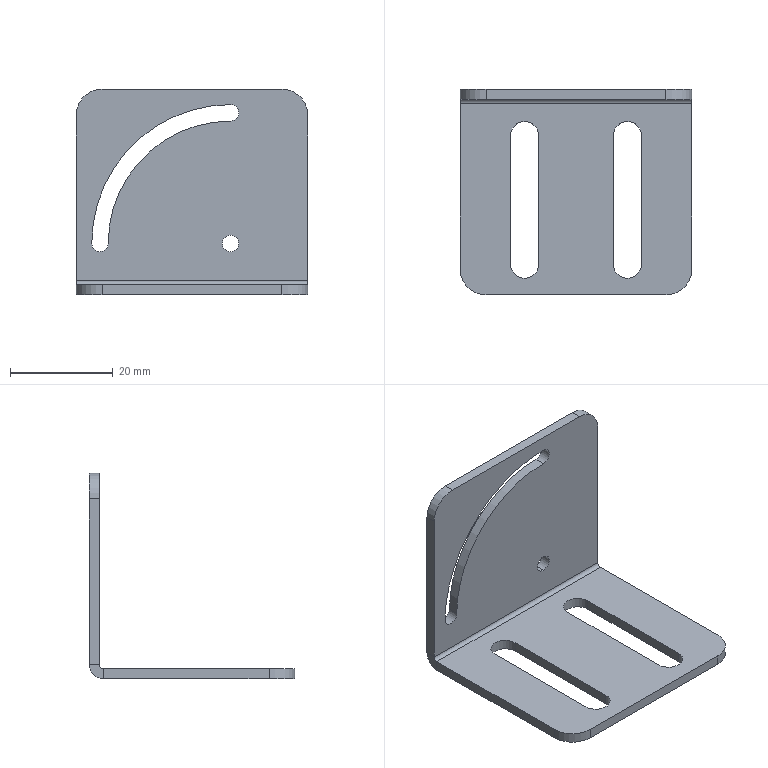Part | SolidWorks | features ICE 2, EdgeFlange 1, Fillet 1, FlatPattern 1, HoleWzd 1, SMBaseFlange 1, SheetMetal 1 | 1 solid | 32 faces | box 45 x 40 x 40 mm | volume 5977 mm3 | cylinder 16 | plane 16 | commonest cylinder face diameters 3.2 x4 5.5 x4 10 x4 1.473 x1 5.473 x1 47.6 x1
STEP:
#1=CARTESIAN_POINT('',(7.5,18.,8.4));
#2=VERTEX_POINT('',#1);
#3=CARTESIAN_POINT('',(7.5,18.,11.6));
#4=VERTEX_POINT('',#3);
#5=CARTESIAN_POINT('',(7.5,18.,10.));
#6=DIRECTION('',(0.,1.,0.));
#7=DIRECTION('',(0.,0.,1.));
#8=AXIS2_PLACEMENT_3D('',#5,#6,#7);
#9=CIRCLE('',#8,1.6);
#10=EDGE_CURVE('',#2,#4,#9,.T.);
#11=ORIENTED_EDGE('',*,*,#10,.F.);
#12=CARTESIAN_POINT('',(7.5,20.,8.4));
#13=VERTEX_POINT('',#12);
#14=CARTESIAN_POINT('',(7.5,20.,8.4));
#15=DIRECTION('',(0.,1.,0.));
#16=VECTOR('',#15,1000.);
#17=LINE('',#14,#16);
#18=EDGE_CURVE('',#2,#13,#17,.T.);
#19=ORIENTED_EDGE('',*,*,#18,.T.);
#20=CARTESIAN_POINT('',(7.5,20.,11.6));
#21=VERTEX_POINT('',#20);
#22=CARTESIAN_POINT('',(7.5,20.,10.));
#23=DIRECTION('',(0.,1.,0.));
#24=DIRECTION('',(0.,0.,1.));
#25=AXIS2_PLACEMENT_3D('',#22,#23,#24);
#26=CIRCLE('',#25,1.6);
#27=EDGE_CURVE('',#13,#21,#26,.T.);
#28=ORIENTED_EDGE('',*,*,#27,.T.);
#29=CARTESIAN_POINT('',(7.5,20.,11.6));
#30=DIRECTION('',(0.,1.,0.));
#31=VECTOR('',#30,1000.);
#32=LINE('',#29,#31);
#33=EDGE_CURVE('',#4,#21,#32,.T.);
#34=ORIENTED_EDGE('',*,*,#33,.F.);
#35=EDGE_LOOP('',(#11,#19,#28,#34));
#36=FACE_OUTER_BOUND('',#35,.T.);
#37=CARTESIAN_POINT('',(7.5,20.,10.));
#38=DIRECTION('',(0.,1.,0.));
#39=DIRECTION('',(0.,0.,1.));
#40=AXIS2_PLACEMENT_3D('',#37,#38,#39);
#41=CYLINDRICAL_SURFACE('',#40,1.6);
#42=ADVANCED_FACE('',(#36),#41,.F.);
#43=CARTESIAN_POINT('',(22.5,-15.,2.));
#44=VERTEX_POINT('',#43);
#45=CARTESIAN_POINT('',(22.5,17.263,2.));
#46=VERTEX_POINT('',#45);
#47=CARTESIAN_POINT('',(22.5,-20.,2.));
#48=DIRECTION('',(0.,1.,0.));
#49=VECTOR('',#48,1000.);
#50=LINE('',#47,#49);
#51=EDGE_CURVE('',#44,#46,#50,.T.);
#52=ORIENTED_EDGE('',*,*,#51,.F.);
#53=CARTESIAN_POINT('',(22.5,-15.,0.));
#54=VERTEX_POINT('',#53);
#55=CARTESIAN_POINT('',(22.5,-15.,2.));
#56=DIRECTION('',(0.,0.,-1.));
#57=VECTOR('',#56,1000.);
#58=LINE('',#55,#57);
#59=EDGE_CURVE('',#44,#54,#58,.T.);
#60=ORIENTED_EDGE('',*,*,#59,.T.);
#61=CARTESIAN_POINT('',(22.5,17.263,0.));
#62=VERTEX_POINT('',#61);
#63=CARTESIAN_POINT('',(22.5,-20.,0.));
#64=DIRECTION('',(0.,1.,0.));
#65=VECTOR('',#64,1000.);
#66=LINE('',#63,#65);
#67=EDGE_CURVE('',#54,#62,#66,.T.);
#68=ORIENTED_EDGE('',*,*,#67,.T.);
#69=CARTESIAN_POINT('',(22.5,17.263,2.));
#70=DIRECTION('',(0.,0.,-1.));
#71=VECTOR('',#70,1000.);
#72=LINE('',#69,#71);
#73=EDGE_CURVE('',#46,#62,#72,.T.);
#74=ORIENTED_EDGE('',*,*,#73,.F.);
#75=EDGE_LOOP('',(#52,#60,#68,#74));
#76=FACE_OUTER_BOUND('',#75,.T.);
#77=CARTESIAN_POINT('',(22.5,-20.,2.));
#78=DIRECTION('',(-1.,0.,0.));
#79=DIRECTION('',(0.,0.,1.));
#80=AXIS2_PLACEMENT_3D('',#77,#78,#79);
#81=PLANE('',#80);
#82=ADVANCED_FACE('',(#76),#81,.F.);
#83=CARTESIAN_POINT('',(-22.5,17.263,0.));
#84=VERTEX_POINT('',#83);
#85=CARTESIAN_POINT('',(-22.5,-15.,0.));
#86=VERTEX_POINT('',#85);
#87=CARTESIAN_POINT('',(-22.5,-20.,0.));
#88=DIRECTION('',(0.,-1.,0.));
#89=VECTOR('',#88,1000.);
#90=LINE('',#87,#89);
#91=EDGE_CURVE('',#84,#86,#90,.T.);
#92=ORIENTED_EDGE('',*,*,#91,.T.);
#93=CARTESIAN_POINT('',(-22.5,-15.,2.));
#94=VERTEX_POINT('',#93);
#95=CARTESIAN_POINT('',(-22.5,-15.,2.));
#96=DIRECTION('',(0.,0.,1.));
#97=VECTOR('',#96,1000.);
#98=LINE('',#95,#97);
#99=EDGE_CURVE('',#86,#94,#98,.T.);
#100=ORIENTED_EDGE('',*,*,#99,.T.);
#101=CARTESIAN_POINT('',(-22.5,17.263,2.));
#102=VERTEX_POINT('',#101);
#103=CARTESIAN_POINT('',(-22.5,-20.,2.));
#104=DIRECTION('',(0.,-1.,0.));
#105=VECTOR('',#104,1000.);
#106=LINE('',#103,#105);
#107=EDGE_CURVE('',#102,#94,#106,.T.);
#108=ORIENTED_EDGE('',*,*,#107,.F.);
#109=CARTESIAN_POINT('',(-22.5,17.263,2.));
#110=DIRECTION('',(0.,0.,-1.));
#111=VECTOR('',#110,1000.);
#112=LINE('',#109,#111);
#113=EDGE_CURVE('',#102,#84,#112,.T.);
#114=ORIENTED_EDGE('',*,*,#113,.T.);
#115=EDGE_LOOP('',(#92,#100,#108,#114));
#116=FACE_OUTER_BOUND('',#115,.T.);
#117=CARTESIAN_POINT('',(-22.5,-20.,2.));
#118=DIRECTION('',(1.,0.,0.));
#119=DIRECTION('',(0.,0.,-1.));
#120=AXIS2_PLACEMENT_3D('',#117,#118,#119);
#121=PLANE('',#120);
#122=ADVANCED_FACE('',(#116),#121,.F.);
#123=CARTESIAN_POINT('',(-12.75,11.,2.));
#124=VERTEX_POINT('',#123);
#125=CARTESIAN_POINT('',(-12.75,-14.,2.));
#126=VERTEX_POINT('',#125);
#127=CARTESIAN_POINT('',(-12.75,11.,2.));
#128=DIRECTION('',(0.,-1.,0.));
#129=VECTOR('',#128,1000.);
#130=LINE('',#127,#129);
#131=EDGE_CURVE('',#124,#126,#130,.T.);
#132=ORIENTED_EDGE('',*,*,#131,.F.);
#133=CARTESIAN_POINT('',(-7.25,11.,2.));
#134=VERTEX_POINT('',#133);
#135=CARTESIAN_POINT('',(-10.,11.,2.));
#136=DIRECTION('',(0.,0.,1.));
#137=DIRECTION('',(1.,0.,0.));
#138=AXIS2_PLACEMENT_3D('',#135,#136,#137);
#139=CIRCLE('',#138,2.75);
#140=EDGE_CURVE('',#134,#124,#139,.T.);
#141=ORIENTED_EDGE('',*,*,#140,.F.);
#142=CARTESIAN_POINT('',(-7.25,-14.,2.));
#143=VERTEX_POINT('',#142);
#144=CARTESIAN_POINT('',(-7.25,11.,2.));
#145=DIRECTION('',(0.,1.,0.));
#146=VECTOR('',#145,1000.);
#147=LINE('',#144,#146);
#148=EDGE_CURVE('',#143,#134,#147,.T.);
#149=ORIENTED_EDGE('',*,*,#148,.F.);
#150=CARTESIAN_POINT('',(-10.,-14.,2.));
#151=DIRECTION('',(0.,0.,1.));
#152=DIRECTION('',(1.,0.,0.));
#153=AXIS2_PLACEMENT_3D('',#150,#151,#152);
#154=CIRCLE('',#153,2.75);
#155=EDGE_CURVE('',#126,#143,#154,.T.);
#156=ORIENTED_EDGE('',*,*,#155,.F.);
#157=EDGE_LOOP('',(#132,#141,#149,#156));
#158=FACE_BOUND('',#157,.T.);
#159=CARTESIAN_POINT('',(7.25,11.,2.));
#160=VERTEX_POINT('',#159);
#161=CARTESIAN_POINT('',(7.25,-14.,2.));
#162=VERTEX_POINT('',#161);
#163=CARTESIAN_POINT('',(7.25,11.,2.));
#164=DIRECTION('',(0.,-1.,0.));
#165=VECTOR('',#164,1000.);
#166=LINE('',#163,#165);
#167=EDGE_CURVE('',#160,#162,#166,.T.);
#168=ORIENTED_EDGE('',*,*,#167,.F.);
#169=CARTESIAN_POINT('',(12.75,11.,2.));
#170=VERTEX_POINT('',#169);
#171=CARTESIAN_POINT('',(10.,11.,2.));
#172=DIRECTION('',(0.,0.,1.));
#173=DIRECTION('',(1.,0.,0.));
#174=AXIS2_PLACEMENT_3D('',#171,#172,#173);
#175=CIRCLE('',#174,2.75);
#176=EDGE_CURVE('',#170,#160,#175,.T.);
#177=ORIENTED_EDGE('',*,*,#176,.F.);
#178=CARTESIAN_POINT('',(12.75,-14.,2.));
#179=VERTEX_POINT('',#178);
#180=CARTESIAN_POINT('',(12.75,11.,2.));
#181=DIRECTION('',(0.,1.,0.));
#182=VECTOR('',#181,1000.);
#183=LINE('',#180,#182);
#184=EDGE_CURVE('',#179,#170,#183,.T.);
#185=ORIENTED_EDGE('',*,*,#184,.F.);
#186=CARTESIAN_POINT('',(10.,-14.,2.));
#187=DIRECTION('',(0.,0.,1.));
#188=DIRECTION('',(1.,0.,0.));
#189=AXIS2_PLACEMENT_3D('',#186,#187,#188);
#190=CIRCLE('',#189,2.75);
#191=EDGE_CURVE('',#162,#179,#190,.T.);
#192=ORIENTED_EDGE('',*,*,#191,.F.);
#193=EDGE_LOOP('',(#168,#177,#185,#192));
#194=FACE_BOUND('',#193,.T.);
#195=ORIENTED_EDGE('',*,*,#107,.T.);
#196=CARTESIAN_POINT('',(-17.5,-20.,2.));
#197=VERTEX_POINT('',#196);
#198=CARTESIAN_POINT('',(-17.5,-15.,2.));
#199=DIRECTION('',(0.,0.,1.));
#200=DIRECTION('',(-1.,0.,0.));
#201=AXIS2_PLACEMENT_3D('',#198,#199,#200);
#202=CIRCLE('',#201,5.);
#203=EDGE_CURVE('',#94,#197,#202,.T.);
#204=ORIENTED_EDGE('',*,*,#203,.T.);
#205=CARTESIAN_POINT('',(17.5,-20.,2.));
#206=VERTEX_POINT('',#205);
#207=CARTESIAN_POINT('',(-22.5,-20.,2.));
#208=DIRECTION('',(1.,0.,0.));
#209=VECTOR('',#208,1000.);
#210=LINE('',#207,#209);
#211=EDGE_CURVE('',#197,#206,#210,.T.);
#212=ORIENTED_EDGE('',*,*,#211,.T.);
#213=CARTESIAN_POINT('',(17.5,-15.,2.));
#214=DIRECTION('',(0.,0.,1.));
#215=DIRECTION('',(-1.,0.,0.));
#216=AXIS2_PLACEMENT_3D('',#213,#214,#215);
#217=CIRCLE('',#216,5.);
#218=EDGE_CURVE('',#206,#44,#217,.T.);
#219=ORIENTED_EDGE('',*,*,#218,.T.);
#220=ORIENTED_EDGE('',*,*,#51,.T.);
#221=CARTESIAN_POINT('',(-22.5,17.263,2.));
#222=DIRECTION('',(1.,0.,0.));
#223=VECTOR('',#222,1000.);
#224=LINE('',#221,#223);
#225=EDGE_CURVE('',#102,#46,#224,.T.);
#226=ORIENTED_EDGE('',*,*,#225,.F.);
#227=EDGE_LOOP('',(#195,#204,#212,#219,#220,#226));
#228=FACE_OUTER_BOUND('',#227,.T.);
#229=CARTESIAN_POINT('',(0.,0.,2.));
#230=DIRECTION('',(0.,0.,-1.));
#231=DIRECTION('',(-1.,0.,0.));
#232=AXIS2_PLACEMENT_3D('',#229,#230,#231);
#233=PLANE('',#232);
#234=ADVANCED_FACE('',(#158,#194,#228),#233,.F.);
#235=CARTESIAN_POINT('',(-7.25,11.,0.));
#236=VERTEX_POINT('',#235);
#237=CARTESIAN_POINT('',(-12.75,11.,0.));
#238=VERTEX_POINT('',#237);
#239=CARTESIAN_POINT('',(-10.,11.,0.));
#240=DIRECTION('',(0.,0.,1.));
#241=DIRECTION('',(1.,0.,0.));
#242=AXIS2_PLACEMENT_3D('',#239,#240,#241);
#243=CIRCLE('',#242,2.75);
#244=EDGE_CURVE('',#236,#238,#243,.T.);
#245=ORIENTED_EDGE('',*,*,#244,.T.);
#246=CARTESIAN_POINT('',(-12.75,-14.,0.));
#247=VERTEX_POINT('',#246);
#248=CARTESIAN_POINT('',(-12.75,11.,0.));
#249=DIRECTION('',(0.,-1.,0.));
#250=VECTOR('',#249,1000.);
#251=LINE('',#248,#250);
#252=EDGE_CURVE('',#238,#247,#251,.T.);
#253=ORIENTED_EDGE('',*,*,#252,.T.);
#254=CARTESIAN_POINT('',(-7.25,-14.,0.));
#255=VERTEX_POINT('',#254);
#256=CARTESIAN_POINT('',(-10.,-14.,0.));
#257=DIRECTION('',(0.,0.,1.));
#258=DIRECTION('',(1.,0.,0.));
#259=AXIS2_PLACEMENT_3D('',#256,#257,#258);
#260=CIRCLE('',#259,2.75);
#261=EDGE_CURVE('',#247,#255,#260,.T.);
#262=ORIENTED_EDGE('',*,*,#261,.T.);
#263=CARTESIAN_POINT('',(-7.25,11.,0.));
#264=DIRECTION('',(0.,1.,0.));
#265=VECTOR('',#264,1000.);
#266=LINE('',#263,#265);
#267=EDGE_CURVE('',#255,#236,#266,.T.);
#268=ORIENTED_EDGE('',*,*,#267,.T.);
#269=EDGE_LOOP('',(#245,#253,#262,#268));
#270=FACE_BOUND('',#269,.T.);
#271=CARTESIAN_POINT('',(12.75,11.,0.));
#272=VERTEX_POINT('',#271);
#273=CARTESIAN_POINT('',(7.25,11.,0.));
#274=VERTEX_POINT('',#273);
#275=CARTESIAN_POINT('',(10.,11.,0.));
#276=DIRECTION('',(0.,0.,1.));
#277=DIRECTION('',(1.,0.,0.));
#278=AXIS2_PLACEMENT_3D('',#275,#276,#277);
#279=CIRCLE('',#278,2.75);
#280=EDGE_CURVE('',#272,#274,#279,.T.);
#281=ORIENTED_EDGE('',*,*,#280,.T.);
#282=CARTESIAN_POINT('',(7.25,-14.,0.));
#283=VERTEX_POINT('',#282);
#284=CARTESIAN_POINT('',(7.25,11.,0.));
#285=DIRECTION('',(0.,-1.,0.));
#286=VECTOR('',#285,1000.);
#287=LINE('',#284,#286);
#288=EDGE_CURVE('',#274,#283,#287,.T.);
#289=ORIENTED_EDGE('',*,*,#288,.T.);
#290=CARTESIAN_POINT('',(12.75,-14.,0.));
#291=VERTEX_POINT('',#290);
#292=CARTESIAN_POINT('',(10.,-14.,0.));
#293=DIRECTION('',(0.,0.,1.));
#294=DIRECTION('',(1.,0.,0.));
#295=AXIS2_PLACEMENT_3D('',#292,#293,#294);
#296=CIRCLE('',#295,2.75);
#297=EDGE_CURVE('',#283,#291,#296,.T.);
#298=ORIENTED_EDGE('',*,*,#297,.T.);
#299=CARTESIAN_POINT('',(12.75,11.,0.));
#300=DIRECTION('',(0.,1.,0.));
#301=VECTOR('',#300,1000.);
#302=LINE('',#299,#301);
#303=EDGE_CURVE('',#291,#272,#302,.T.);
#304=ORIENTED_EDGE('',*,*,#303,.T.);
#305=EDGE_LOOP('',(#281,#289,#298,#304));
#306=FACE_BOUND('',#305,.T.);
#307=CARTESIAN_POINT('',(-17.5,-20.,0.));
#308=VERTEX_POINT('',#307);
#309=CARTESIAN_POINT('',(17.5,-20.,0.));
#310=VERTEX_POINT('',#309);
#311=CARTESIAN_POINT('',(-22.5,-20.,0.));
#312=DIRECTION('',(1.,0.,0.));
#313=VECTOR('',#312,1000.);
#314=LINE('',#311,#313);
#315=EDGE_CURVE('',#308,#310,#314,.T.);
#316=ORIENTED_EDGE('',*,*,#315,.F.);
#317=CARTESIAN_POINT('',(-17.5,-15.,0.));
#318=DIRECTION('',(0.,0.,-1.));
#319=DIRECTION('',(-1.,0.,0.));
#320=AXIS2_PLACEMENT_3D('',#317,#318,#319);
#321=CIRCLE('',#320,5.);
#322=EDGE_CURVE('',#308,#86,#321,.T.);
#323=ORIENTED_EDGE('',*,*,#322,.T.);
#324=ORIENTED_EDGE('',*,*,#91,.F.);
#325=CARTESIAN_POINT('',(-22.5,17.263,0.));
#326=DIRECTION('',(1.,0.,0.));
#327=VECTOR('',#326,1000.);
#328=LINE('',#325,#327);
#329=EDGE_CURVE('',#84,#62,#328,.T.);
#330=ORIENTED_EDGE('',*,*,#329,.T.);
#331=ORIENTED_EDGE('',*,*,#67,.F.);
#332=CARTESIAN_POINT('',(17.5,-15.,0.));
#333=DIRECTION('',(0.,0.,-1.));
#334=DIRECTION('',(-1.,0.,0.));
#335=AXIS2_PLACEMENT_3D('',#332,#333,#334);
#336=CIRCLE('',#335,5.);
#337=EDGE_CURVE('',#54,#310,#336,.T.);
#338=ORIENTED_EDGE('',*,*,#337,.T.);
#339=EDGE_LOOP('',(#316,#323,#324,#330,#331,#338));
#340=FACE_OUTER_BOUND('',#339,.T.);
#341=CARTESIAN_POINT('',(0.,0.,0.));
#342=DIRECTION('',(0.,0.,-1.));
#343=DIRECTION('',(-1.,0.,0.));
#344=AXIS2_PLACEMENT_3D('',#341,#342,#343);
#345=PLANE('',#344);
#346=ADVANCED_FACE('',(#270,#306,#340),#345,.T.);
#347=ORIENTED_EDGE('',*,*,#211,.F.);
#348=CARTESIAN_POINT('',(-17.5,-20.,2.));
#349=DIRECTION('',(0.,0.,-1.));
#350=VECTOR('',#349,1000.);
#351=LINE('',#348,#350);
#352=EDGE_CURVE('',#197,#308,#351,.T.);
#353=ORIENTED_EDGE('',*,*,#352,.T.);
#354=ORIENTED_EDGE('',*,*,#315,.T.);
#355=CARTESIAN_POINT('',(17.5,-20.,2.));
#356=DIRECTION('',(0.,0.,1.));
#357=VECTOR('',#356,1000.);
#358=LINE('',#355,#357);
#359=EDGE_CURVE('',#310,#206,#358,.T.);
#360=ORIENTED_EDGE('',*,*,#359,.T.);
#361=EDGE_LOOP('',(#347,#353,#354,#360));
#362=FACE_OUTER_BOUND('',#361,.T.);
#363=CARTESIAN_POINT('',(-22.5,-20.,2.));
#364=DIRECTION('',(0.,1.,0.));
#365=DIRECTION('',(0.,0.,1.));
#366=AXIS2_PLACEMENT_3D('',#363,#364,#365);
#367=PLANE('',#366);
#368=ADVANCED_FACE('',(#362),#367,.F.);
#369=CARTESIAN_POINT('',(22.5,18.,2.737));
#370=VERTEX_POINT('',#369);
#371=CARTESIAN_POINT('',(22.5,20.,2.737));
#372=VERTEX_POINT('',#371);
#373=CARTESIAN_POINT('',(22.5,20.,2.737));
#374=DIRECTION('',(0.,1.,0.));
#375=VECTOR('',#374,1000.);
#376=LINE('',#373,#375);
#377=EDGE_CURVE('',#370,#372,#376,.T.);
#378=ORIENTED_EDGE('',*,*,#377,.F.);
#379=CARTESIAN_POINT('',(22.5,17.263,2.737));
#380=DIRECTION('',(1.,0.,0.));
#381=DIRECTION('',(0.,0.,1.));
#382=AXIS2_PLACEMENT_3D('',#379,#380,#381);
#383=CIRCLE('',#382,0.7366);
#384=EDGE_CURVE('',#46,#370,#383,.T.);
#385=ORIENTED_EDGE('',*,*,#384,.F.);
#386=ORIENTED_EDGE('',*,*,#73,.T.);
#387=CARTESIAN_POINT('',(22.5,17.263,2.737));
#388=DIRECTION('',(1.,0.,0.));
#389=DIRECTION('',(0.,0.,1.));
#390=AXIS2_PLACEMENT_3D('',#387,#388,#389);
#391=CIRCLE('',#390,2.737);
#392=EDGE_CURVE('',#62,#372,#391,.T.);
#393=ORIENTED_EDGE('',*,*,#392,.T.);
#394=EDGE_LOOP('',(#378,#385,#386,#393));
#395=FACE_OUTER_BOUND('',#394,.T.);
#396=CARTESIAN_POINT('',(22.5,17.263,2.737));
#397=DIRECTION('',(1.,0.,0.));
#398=DIRECTION('',(0.,0.,-1.));
#399=AXIS2_PLACEMENT_3D('',#396,#397,#398);
#400=PLANE('',#399);
#401=ADVANCED_FACE('',(#395),#400,.T.);
#402=CARTESIAN_POINT('',(-22.5,18.,2.737));
#403=VERTEX_POINT('',#402);
#404=CARTESIAN_POINT('',(-22.5,17.263,2.737));
#405=DIRECTION('',(-1.,0.,0.));
#406=DIRECTION('',(0.,0.,1.));
#407=AXIS2_PLACEMENT_3D('',#404,#405,#406);
#408=CIRCLE('',#407,0.7366);
#409=EDGE_CURVE('',#403,#102,#408,.T.);
#410=ORIENTED_EDGE('',*,*,#409,.F.);
#411=CARTESIAN_POINT('',(-22.5,20.,2.737));
#412=VERTEX_POINT('',#411);
#413=CARTESIAN_POINT('',(-22.5,18.,2.737));
#414=DIRECTION('',(0.,1.,0.));
#415=VECTOR('',#414,1000.);
#416=LINE('',#413,#415);
#417=EDGE_CURVE('',#403,#412,#416,.T.);
#418=ORIENTED_EDGE('',*,*,#417,.T.);
#419=CARTESIAN_POINT('',(-22.5,17.263,2.737));
#420=DIRECTION('',(-1.,0.,0.));
#421=DIRECTION('',(0.,0.,1.));
#422=AXIS2_PLACEMENT_3D('',#419,#420,#421);
#423=CIRCLE('',#422,2.737);
#424=EDGE_CURVE('',#412,#84,#423,.T.);
#425=ORIENTED_EDGE('',*,*,#424,.T.);
#426=ORIENTED_EDGE('',*,*,#113,.F.);
#427=EDGE_LOOP('',(#410,#418,#425,#426));
#428=FACE_OUTER_BOUND('',#427,.T.);
#429=CARTESIAN_POINT('',(-22.5,17.263,2.737));
#430=DIRECTION('',(1.,0.,0.));
#431=DIRECTION('',(0.,0.,-1.));
#432=AXIS2_PLACEMENT_3D('',#429,#430,#431);
#433=PLANE('',#432);
#434=ADVANCED_FACE('',(#428),#433,.F.);
#435=ORIENTED_EDGE('',*,*,#329,.F.);
#436=ORIENTED_EDGE('',*,*,#424,.F.);
#437=CARTESIAN_POINT('',(0.,20.,2.737));
#438=DIRECTION('',(-1.,0.,0.));
#439=VECTOR('',#438,1000.);
#440=LINE('',#437,#439);
#441=EDGE_CURVE('',#372,#412,#440,.T.);
#442=ORIENTED_EDGE('',*,*,#441,.F.);
#443=ORIENTED_EDGE('',*,*,#392,.F.);
#444=EDGE_LOOP('',(#435,#436,#442,#443));
#445=FACE_OUTER_BOUND('',#444,.T.);
#446=CARTESIAN_POINT('',(-22.5,17.263,2.737));
#447=DIRECTION('',(-1.,0.,0.));
#448=DIRECTION('',(0.,1.,0.));
#449=AXIS2_PLACEMENT_3D('',#446,#447,#448);
#450=CYLINDRICAL_SURFACE('',#449,2.737);
#451=ADVANCED_FACE('',(#445),#450,.T.);
#452=ORIENTED_EDGE('',*,*,#225,.T.);
#453=ORIENTED_EDGE('',*,*,#384,.T.);
#454=CARTESIAN_POINT('',(22.5,18.,2.737));
#455=DIRECTION('',(-1.,0.,0.));
#456=VECTOR('',#455,1000.);
#457=LINE('',#454,#456);
#458=EDGE_CURVE('',#370,#403,#457,.T.);
#459=ORIENTED_EDGE('',*,*,#458,.T.);
#460=ORIENTED_EDGE('',*,*,#409,.T.);
#461=EDGE_LOOP('',(#452,#453,#459,#460));
#462=FACE_OUTER_BOUND('',#461,.T.);
#463=CARTESIAN_POINT('',(-22.5,17.263,2.737));
#464=DIRECTION('',(-1.,0.,0.));
#465=DIRECTION('',(0.,1.,0.));
#466=AXIS2_PLACEMENT_3D('',#463,#464,#465);
#467=CYLINDRICAL_SURFACE('',#466,0.7366);
#468=ADVANCED_FACE('',(#462),#467,.F.);
#469=CARTESIAN_POINT('',(-22.5,18.,35.));
#470=VERTEX_POINT('',#469);
#471=CARTESIAN_POINT('',(-22.5,18.,0.));
#472=DIRECTION('',(0.,0.,-1.));
#473=VECTOR('',#472,1000.);
#474=LINE('',#471,#473);
#475=EDGE_CURVE('',#470,#403,#474,.T.);
#476=ORIENTED_EDGE('',*,*,#475,.F.);
#477=CARTESIAN_POINT('',(-22.5,20.,35.));
#478=VERTEX_POINT('',#477);
#479=CARTESIAN_POINT('',(-22.5,20.,35.));
#480=DIRECTION('',(0.,1.,0.));
#481=VECTOR('',#480,1000.);
#482=LINE('',#479,#481);
#483=EDGE_CURVE('',#470,#478,#482,.T.);
#484=ORIENTED_EDGE('',*,*,#483,.T.);
#485=CARTESIAN_POINT('',(-22.5,20.,2.));
#486=DIRECTION('',(0.,0.,-1.));
#487=VECTOR('',#486,1000.);
#488=LINE('',#485,#487);
#489=EDGE_CURVE('',#478,#412,#488,.T.);
#490=ORIENTED_EDGE('',*,*,#489,.T.);
#491=ORIENTED_EDGE('',*,*,#417,.F.);
#492=EDGE_LOOP('',(#476,#484,#490,#491));
#493=FACE_OUTER_BOUND('',#492,.T.);
#494=CARTESIAN_POINT('',(-22.5,20.,2.));
#495=DIRECTION('',(-1.,0.,0.));
#496=DIRECTION('',(0.,0.,1.));
#497=AXIS2_PLACEMENT_3D('',#494,#495,#496);
#498=PLANE('',#497);
#499=ADVANCED_FACE('',(#493),#498,.T.);
#500=CARTESIAN_POINT('',(22.5,20.,35.));
#501=VERTEX_POINT('',#500);
#502=CARTESIAN_POINT('',(22.5,20.,40.));
#503=DIRECTION('',(0.,0.,1.));
#504=VECTOR('',#503,1000.);
#505=LINE('',#502,#504);
#506=EDGE_CURVE('',#372,#501,#505,.T.);
#507=ORIENTED_EDGE('',*,*,#506,.T.);
#508=CARTESIAN_POINT('',(22.5,18.,35.));
#509=VERTEX_POINT('',#508);
#510=CARTESIAN_POINT('',(22.5,20.,35.));
#511=DIRECTION('',(0.,-1.,0.));
#512=VECTOR('',#511,1000.);
#513=LINE('',#510,#512);
#514=EDGE_CURVE('',#501,#509,#513,.T.);
#515=ORIENTED_EDGE('',*,*,#514,.T.);
#516=CARTESIAN_POINT('',(22.5,18.,0.));
#517=DIRECTION('',(0.,0.,1.));
#518=VECTOR('',#517,1000.);
#519=LINE('',#516,#518);
#520=EDGE_CURVE('',#370,#509,#519,.T.);
#521=ORIENTED_EDGE('',*,*,#520,.F.);
#522=ORIENTED_EDGE('',*,*,#377,.T.);
#523=EDGE_LOOP('',(#507,#515,#521,#522));
#524=FACE_OUTER_BOUND('',#523,.T.);
#525=CARTESIAN_POINT('',(22.5,20.,40.));
#526=DIRECTION('',(1.,0.,0.));
#527=DIRECTION('',(0.,0.,-1.));
#528=AXIS2_PLACEMENT_3D('',#525,#526,#527);
#529=PLANE('',#528);
#530=ADVANCED_FACE('',(#524),#529,.T.);
#531=CARTESIAN_POINT('',(-16.3,20.,10.));
#532=VERTEX_POINT('',#531);
#533=CARTESIAN_POINT('',(-19.5,20.,10.));
#534=VERTEX_POINT('',#533);
#535=CARTESIAN_POINT('',(-17.9,20.,10.));
#536=DIRECTION('',(0.,1.,0.));
#537=DIRECTION('',(0.,0.,1.));
#538=AXIS2_PLACEMENT_3D('',#535,#536,#537);
#539=CIRCLE('',#538,1.6);
#540=EDGE_CURVE('',#532,#534,#539,.T.);
#541=ORIENTED_EDGE('',*,*,#540,.F.);
#542=CARTESIAN_POINT('',(7.5,20.,33.8));
#543=VERTEX_POINT('',#542);
#544=CARTESIAN_POINT('',(7.5,20.,10.));
#545=DIRECTION('',(0.,-1.,0.));
#546=DIRECTION('',(0.,0.,1.));
#547=AXIS2_PLACEMENT_3D('',#544,#545,#546);
#548=CIRCLE('',#547,23.8);
#549=EDGE_CURVE('',#543,#532,#548,.T.);
#550=ORIENTED_EDGE('',*,*,#549,.F.);
#551=CARTESIAN_POINT('',(7.5,20.,37.));
#552=VERTEX_POINT('',#551);
#553=CARTESIAN_POINT('',(7.5,20.,35.4));
#554=DIRECTION('',(0.,1.,0.));
#555=DIRECTION('',(0.,0.,1.));
#556=AXIS2_PLACEMENT_3D('',#553,#554,#555);
#557=CIRCLE('',#556,1.6);
#558=EDGE_CURVE('',#552,#543,#557,.T.);
#559=ORIENTED_EDGE('',*,*,#558,.F.);
#560=CARTESIAN_POINT('',(7.5,20.,10.));
#561=DIRECTION('',(0.,1.,0.));
#562=DIRECTION('',(0.,0.,1.));
#563=AXIS2_PLACEMENT_3D('',#560,#561,#562);
#564=CIRCLE('',#563,27.);
#565=EDGE_CURVE('',#534,#552,#564,.T.);
#566=ORIENTED_EDGE('',*,*,#565,.F.);
#567=EDGE_LOOP('',(#541,#550,#559,#566));
#568=FACE_BOUND('',#567,.T.);
#569=CARTESIAN_POINT('',(7.5,20.,10.));
#570=DIRECTION('',(0.,1.,0.));
#571=DIRECTION('',(0.,0.,1.));
#572=AXIS2_PLACEMENT_3D('',#569,#570,#571);
#573=CIRCLE('',#572,1.6);
#574=EDGE_CURVE('',#21,#13,#573,.T.);
#575=ORIENTED_EDGE('',*,*,#574,.F.);
#576=ORIENTED_EDGE('',*,*,#27,.F.);
#577=EDGE_LOOP('',(#575,#576));
#578=FACE_BOUND('',#577,.T.);
#579=CARTESIAN_POINT('',(17.5,20.,40.));
#580=VERTEX_POINT('',#579);
#581=CARTESIAN_POINT('',(-17.5,20.,40.));
#582=VERTEX_POINT('',#581);
#583=CARTESIAN_POINT('',(-22.5,20.,40.));
#584=DIRECTION('',(-1.,0.,0.));
#585=VECTOR('',#584,1000.);
#586=LINE('',#583,#585);
#587=EDGE_CURVE('',#580,#582,#586,.T.);
#588=ORIENTED_EDGE('',*,*,#587,.F.);
#589=CARTESIAN_POINT('',(17.5,20.,35.));
#590=DIRECTION('',(0.,1.,0.));
#591=DIRECTION('',(0.,0.,1.));
#592=AXIS2_PLACEMENT_3D('',#589,#590,#591);
#593=CIRCLE('',#592,5.);
#594=EDGE_CURVE('',#580,#501,#593,.T.);
#595=ORIENTED_EDGE('',*,*,#594,.T.);
#596=ORIENTED_EDGE('',*,*,#506,.F.);
#597=ORIENTED_EDGE('',*,*,#441,.T.);
#598=ORIENTED_EDGE('',*,*,#489,.F.);
#599=CARTESIAN_POINT('',(-17.5,20.,35.));
#600=DIRECTION('',(0.,1.,0.));
#601=DIRECTION('',(0.,0.,1.));
#602=AXIS2_PLACEMENT_3D('',#599,#600,#601);
#603=CIRCLE('',#602,5.);
#604=EDGE_CURVE('',#478,#582,#603,.T.);
#605=ORIENTED_EDGE('',*,*,#604,.T.);
#606=EDGE_LOOP('',(#588,#595,#596,#597,#598,#605));
#607=FACE_OUTER_BOUND('',#606,.T.);
#608=CARTESIAN_POINT('',(0.,20.,0.));
#609=DIRECTION('',(0.,1.,0.));
#610=DIRECTION('',(0.,0.,1.));
#611=AXIS2_PLACEMENT_3D('',#608,#609,#610);
#612=PLANE('',#611);
#613=ADVANCED_FACE('',(#568,#578,#607),#612,.T.);
#614=CARTESIAN_POINT('',(-16.3,18.,10.));
#615=VERTEX_POINT('',#614);
#616=CARTESIAN_POINT('',(7.5,18.,33.8));
#617=VERTEX_POINT('',#616);
#618=CARTESIAN_POINT('',(7.5,18.,10.));
#619=DIRECTION('',(0.,1.,0.));
#620=DIRECTION('',(0.,0.,1.));
#621=AXIS2_PLACEMENT_3D('',#618,#619,#620);
#622=CIRCLE('',#621,23.8);
#623=EDGE_CURVE('',#615,#617,#622,.T.);
#624=ORIENTED_EDGE('',*,*,#623,.F.);
#625=CARTESIAN_POINT('',(-19.5,18.,10.));
#626=VERTEX_POINT('',#625);
#627=CARTESIAN_POINT('',(-17.9,18.,10.));
#628=DIRECTION('',(0.,-1.,0.));
#629=DIRECTION('',(0.,0.,1.));
#630=AXIS2_PLACEMENT_3D('',#627,#628,#629);
#631=CIRCLE('',#630,1.6);
#632=EDGE_CURVE('',#626,#615,#631,.T.);
#633=ORIENTED_EDGE('',*,*,#632,.F.);
#634=CARTESIAN_POINT('',(7.5,18.,37.));
#635=VERTEX_POINT('',#634);
#636=CARTESIAN_POINT('',(7.5,18.,10.));
#637=DIRECTION('',(0.,-1.,0.));
#638=DIRECTION('',(0.,0.,1.));
#639=AXIS2_PLACEMENT_3D('',#636,#637,#638);
#640=CIRCLE('',#639,27.);
#641=EDGE_CURVE('',#635,#626,#640,.T.);
#642=ORIENTED_EDGE('',*,*,#641,.F.);
#643=CARTESIAN_POINT('',(7.5,18.,35.4));
#644=DIRECTION('',(0.,-1.,0.));
#645=DIRECTION('',(0.,0.,1.));
#646=AXIS2_PLACEMENT_3D('',#643,#644,#645);
#647=CIRCLE('',#646,1.6);
#648=EDGE_CURVE('',#617,#635,#647,.T.);
#649=ORIENTED_EDGE('',*,*,#648,.F.);
#650=EDGE_LOOP('',(#624,#633,#642,#649));
#651=FACE_BOUND('',#650,.T.);
#652=CARTESIAN_POINT('',(7.5,18.,10.));
#653=DIRECTION('',(0.,1.,0.));
#654=DIRECTION('',(0.,0.,1.));
#655=AXIS2_PLACEMENT_3D('',#652,#653,#654);
#656=CIRCLE('',#655,1.6);
#657=EDGE_CURVE('',#4,#2,#656,.T.);
#658=ORIENTED_EDGE('',*,*,#657,.T.);
#659=ORIENTED_EDGE('',*,*,#10,.T.);
#660=EDGE_LOOP('',(#658,#659));
#661=FACE_BOUND('',#660,.T.);
#662=ORIENTED_EDGE('',*,*,#520,.T.);
#663=CARTESIAN_POINT('',(17.5,18.,40.));
#664=VERTEX_POINT('',#663);
#665=CARTESIAN_POINT('',(17.5,18.,35.));
#666=DIRECTION('',(0.,-1.,0.));
#667=DIRECTION('',(0.,0.,1.));
#668=AXIS2_PLACEMENT_3D('',#665,#666,#667);
#669=CIRCLE('',#668,5.);
#670=EDGE_CURVE('',#509,#664,#669,.T.);
#671=ORIENTED_EDGE('',*,*,#670,.T.);
#672=CARTESIAN_POINT('',(-17.5,18.,40.));
#673=VERTEX_POINT('',#672);
#674=CARTESIAN_POINT('',(0.,18.,40.));
#675=DIRECTION('',(-1.,0.,0.));
#676=VECTOR('',#675,1000.);
#677=LINE('',#674,#676);
#678=EDGE_CURVE('',#664,#673,#677,.T.);
#679=ORIENTED_EDGE('',*,*,#678,.T.);
#680=CARTESIAN_POINT('',(-17.5,18.,35.));
#681=DIRECTION('',(0.,-1.,0.));
#682=DIRECTION('',(0.,0.,1.));
#683=AXIS2_PLACEMENT_3D('',#680,#681,#682);
#684=CIRCLE('',#683,5.);
#685=EDGE_CURVE('',#673,#470,#684,.T.);
#686=ORIENTED_EDGE('',*,*,#685,.T.);
#687=ORIENTED_EDGE('',*,*,#475,.T.);
#688=ORIENTED_EDGE('',*,*,#458,.F.);
#689=EDGE_LOOP('',(#662,#671,#679,#686,#687,#688));
#690=FACE_OUTER_BOUND('',#689,.T.);
#691=CARTESIAN_POINT('',(0.,18.,0.));
#692=DIRECTION('',(0.,1.,0.));
#693=DIRECTION('',(0.,0.,1.));
#694=AXIS2_PLACEMENT_3D('',#691,#692,#693);
#695=PLANE('',#694);
#696=ADVANCED_FACE('',(#651,#661,#690),#695,.F.);
#697=ORIENTED_EDGE('',*,*,#678,.F.);
#698=CARTESIAN_POINT('',(17.5,20.,40.));
#699=DIRECTION('',(0.,1.,0.));
#700=VECTOR('',#699,1000.);
#701=LINE('',#698,#700);
#702=EDGE_CURVE('',#664,#580,#701,.T.);
#703=ORIENTED_EDGE('',*,*,#702,.T.);
#704=ORIENTED_EDGE('',*,*,#587,.T.);
#705=CARTESIAN_POINT('',(-17.5,20.,40.));
#706=DIRECTION('',(0.,-1.,0.));
#707=VECTOR('',#706,1000.);
#708=LINE('',#705,#707);
#709=EDGE_CURVE('',#582,#673,#708,.T.);
#710=ORIENTED_EDGE('',*,*,#709,.T.);
#711=EDGE_LOOP('',(#697,#703,#704,#710));
#712=FACE_OUTER_BOUND('',#711,.T.);
#713=CARTESIAN_POINT('',(-22.5,20.,40.));
#714=DIRECTION('',(0.,0.,1.));
#715=DIRECTION('',(0.,-1.,0.));
#716=AXIS2_PLACEMENT_3D('',#713,#714,#715);
#717=PLANE('',#716);
#718=ADVANCED_FACE('',(#712),#717,.T.);
#719=ORIENTED_EDGE('',*,*,#176,.T.);
#720=CARTESIAN_POINT('',(7.25,11.,0.));
#721=DIRECTION('',(0.,0.,1.));
#722=VECTOR('',#721,1000.);
#723=LINE('',#720,#722);
#724=EDGE_CURVE('',#274,#160,#723,.T.);
#725=ORIENTED_EDGE('',*,*,#724,.F.);
#726=ORIENTED_EDGE('',*,*,#280,.F.);
#727=CARTESIAN_POINT('',(12.75,11.,0.));
#728=DIRECTION('',(0.,0.,1.));
#729=VECTOR('',#728,1000.);
#730=LINE('',#727,#729);
#731=EDGE_CURVE('',#272,#170,#730,.T.);
#732=ORIENTED_EDGE('',*,*,#731,.T.);
#733=EDGE_LOOP('',(#719,#725,#726,#732));
#734=FACE_OUTER_BOUND('',#733,.T.);
#735=CARTESIAN_POINT('',(10.,11.,0.));
#736=DIRECTION('',(0.,0.,1.));
#737=DIRECTION('',(1.,0.,0.));
#738=AXIS2_PLACEMENT_3D('',#735,#736,#737);
#739=CYLINDRICAL_SURFACE('',#738,2.75);
#740=ADVANCED_FACE('',(#734),#739,.F.);
#741=ORIENTED_EDGE('',*,*,#184,.T.);
#742=ORIENTED_EDGE('',*,*,#731,.F.);
#743=ORIENTED_EDGE('',*,*,#303,.F.);
#744=CARTESIAN_POINT('',(12.75,-14.,0.));
#745=DIRECTION('',(0.,0.,1.));
#746=VECTOR('',#745,1000.);
#747=LINE('',#744,#746);
#748=EDGE_CURVE('',#291,#179,#747,.T.);
#749=ORIENTED_EDGE('',*,*,#748,.T.);
#750=EDGE_LOOP('',(#741,#742,#743,#749));
#751=FACE_OUTER_BOUND('',#750,.T.);
#752=CARTESIAN_POINT('',(12.75,11.,0.));
#753=DIRECTION('',(1.,0.,0.));
#754=DIRECTION('',(0.,1.,0.));
#755=AXIS2_PLACEMENT_3D('',#752,#753,#754);
#756=PLANE('',#755);
#757=ADVANCED_FACE('',(#751),#756,.F.);
#758=ORIENTED_EDGE('',*,*,#191,.T.);
#759=ORIENTED_EDGE('',*,*,#748,.F.);
#760=ORIENTED_EDGE('',*,*,#297,.F.);
#761=CARTESIAN_POINT('',(7.25,-14.,0.));
#762=DIRECTION('',(0.,0.,1.));
#763=VECTOR('',#762,1000.);
#764=LINE('',#761,#763);
#765=EDGE_CURVE('',#283,#162,#764,.T.);
#766=ORIENTED_EDGE('',*,*,#765,.T.);
#767=EDGE_LOOP('',(#758,#759,#760,#766));
#768=FACE_OUTER_BOUND('',#767,.T.);
#769=CARTESIAN_POINT('',(10.,-14.,0.));
#770=DIRECTION('',(0.,0.,1.));
#771=DIRECTION('',(1.,0.,0.));
#772=AXIS2_PLACEMENT_3D('',#769,#770,#771);
#773=CYLINDRICAL_SURFACE('',#772,2.75);
#774=ADVANCED_FACE('',(#768),#773,.F.);
#775=ORIENTED_EDGE('',*,*,#167,.T.);
#776=ORIENTED_EDGE('',*,*,#765,.F.);
#777=ORIENTED_EDGE('',*,*,#288,.F.);
#778=ORIENTED_EDGE('',*,*,#724,.T.);
#779=EDGE_LOOP('',(#775,#776,#777,#778));
#780=FACE_OUTER_BOUND('',#779,.T.);
#781=CARTESIAN_POINT('',(7.25,11.,0.));
#782=DIRECTION('',(-1.,0.,0.));
#783=DIRECTION('',(0.,-1.,0.));
#784=AXIS2_PLACEMENT_3D('',#781,#782,#783);
#785=PLANE('',#784);
#786=ADVANCED_FACE('',(#780),#785,.F.);
#787=ORIENTED_EDGE('',*,*,#140,.T.);
#788=CARTESIAN_POINT('',(-12.75,11.,0.));
#789=DIRECTION('',(0.,0.,1.));
#790=VECTOR('',#789,1000.);
#791=LINE('',#788,#790);
#792=EDGE_CURVE('',#238,#124,#791,.T.);
#793=ORIENTED_EDGE('',*,*,#792,.F.);
#794=ORIENTED_EDGE('',*,*,#244,.F.);
#795=CARTESIAN_POINT('',(-7.25,11.,0.));
#796=DIRECTION('',(0.,0.,1.));
#797=VECTOR('',#796,1000.);
#798=LINE('',#795,#797);
#799=EDGE_CURVE('',#236,#134,#798,.T.);
#800=ORIENTED_EDGE('',*,*,#799,.T.);
#801=EDGE_LOOP('',(#787,#793,#794,#800));
#802=FACE_OUTER_BOUND('',#801,.T.);
#803=CARTESIAN_POINT('',(-10.,11.,0.));
#804=DIRECTION('',(0.,0.,1.));
#805=DIRECTION('',(1.,0.,0.));
#806=AXIS2_PLACEMENT_3D('',#803,#804,#805);
#807=CYLINDRICAL_SURFACE('',#806,2.75);
#808=ADVANCED_FACE('',(#802),#807,.F.);
#809=ORIENTED_EDGE('',*,*,#148,.T.);
#810=ORIENTED_EDGE('',*,*,#799,.F.);
#811=ORIENTED_EDGE('',*,*,#267,.F.);
#812=CARTESIAN_POINT('',(-7.25,-14.,0.));
#813=DIRECTION('',(0.,0.,1.));
#814=VECTOR('',#813,1000.);
#815=LINE('',#812,#814);
#816=EDGE_CURVE('',#255,#143,#815,.T.);
#817=ORIENTED_EDGE('',*,*,#816,.T.);
#818=EDGE_LOOP('',(#809,#810,#811,#817));
#819=FACE_OUTER_BOUND('',#818,.T.);
#820=CARTESIAN_POINT('',(-7.25,11.,0.));
#821=DIRECTION('',(1.,0.,0.));
#822=DIRECTION('',(0.,1.,0.));
#823=AXIS2_PLACEMENT_3D('',#820,#821,#822);
#824=PLANE('',#823);
#825=ADVANCED_FACE('',(#819),#824,.F.);
#826=ORIENTED_EDGE('',*,*,#155,.T.);
#827=ORIENTED_EDGE('',*,*,#816,.F.);
#828=ORIENTED_EDGE('',*,*,#261,.F.);
#829=CARTESIAN_POINT('',(-12.75,-14.,0.));
#830=DIRECTION('',(0.,0.,1.));
#831=VECTOR('',#830,1000.);
#832=LINE('',#829,#831);
#833=EDGE_CURVE('',#247,#126,#832,.T.);
#834=ORIENTED_EDGE('',*,*,#833,.T.);
#835=EDGE_LOOP('',(#826,#827,#828,#834));
#836=FACE_OUTER_BOUND('',#835,.T.);
#837=CARTESIAN_POINT('',(-10.,-14.,0.));
#838=DIRECTION('',(0.,0.,1.));
#839=DIRECTION('',(1.,0.,0.));
#840=AXIS2_PLACEMENT_3D('',#837,#838,#839);
#841=CYLINDRICAL_SURFACE('',#840,2.75);
#842=ADVANCED_FACE('',(#836),#841,.F.);
#843=ORIENTED_EDGE('',*,*,#131,.T.);
#844=ORIENTED_EDGE('',*,*,#833,.F.);
#845=ORIENTED_EDGE('',*,*,#252,.F.);
#846=ORIENTED_EDGE('',*,*,#792,.T.);
#847=EDGE_LOOP('',(#843,#844,#845,#846));
#848=FACE_OUTER_BOUND('',#847,.T.);
#849=CARTESIAN_POINT('',(-12.75,11.,0.));
#850=DIRECTION('',(-1.,0.,0.));
#851=DIRECTION('',(0.,-1.,0.));
#852=AXIS2_PLACEMENT_3D('',#849,#850,#851);
#853=PLANE('',#852);
#854=ADVANCED_FACE('',(#848),#853,.F.);
#855=ORIENTED_EDGE('',*,*,#18,.F.);
#856=ORIENTED_EDGE('',*,*,#657,.F.);
#857=ORIENTED_EDGE('',*,*,#33,.T.);
#858=ORIENTED_EDGE('',*,*,#574,.T.);
#859=EDGE_LOOP('',(#855,#856,#857,#858));
#860=FACE_OUTER_BOUND('',#859,.T.);
#861=CARTESIAN_POINT('',(7.5,20.,10.));
#862=DIRECTION('',(0.,1.,0.));
#863=DIRECTION('',(0.,0.,1.));
#864=AXIS2_PLACEMENT_3D('',#861,#862,#863);
#865=CYLINDRICAL_SURFACE('',#864,1.6);
#866=ADVANCED_FACE('',(#860),#865,.F.);
#867=ORIENTED_EDGE('',*,*,#632,.T.);
#868=CARTESIAN_POINT('',(-16.3,-22.447,10.));
#869=DIRECTION('',(0.,1.,0.));
#870=VECTOR('',#869,1000.);
#871=LINE('',#868,#870);
#872=EDGE_CURVE('',#615,#532,#871,.T.);
#873=ORIENTED_EDGE('',*,*,#872,.T.);
#874=ORIENTED_EDGE('',*,*,#540,.T.);
#875=CARTESIAN_POINT('',(-19.5,-22.447,10.));
#876=DIRECTION('',(0.,1.,0.));
#877=VECTOR('',#876,1000.);
#878=LINE('',#875,#877);
#879=EDGE_CURVE('',#626,#534,#878,.T.);
#880=ORIENTED_EDGE('',*,*,#879,.F.);
#881=EDGE_LOOP('',(#867,#873,#874,#880));
#882=FACE_OUTER_BOUND('',#881,.T.);
#883=CARTESIAN_POINT('',(-17.9,-22.447,10.));
#884=DIRECTION('',(0.,1.,0.));
#885=DIRECTION('',(0.,0.,1.));
#886=AXIS2_PLACEMENT_3D('',#883,#884,#885);
#887=CYLINDRICAL_SURFACE('',#886,1.6);
#888=ADVANCED_FACE('',(#882),#887,.F.);
#889=ORIENTED_EDGE('',*,*,#623,.T.);
#890=CARTESIAN_POINT('',(7.5,-22.447,33.8));
#891=DIRECTION('',(0.,1.,0.));
#892=VECTOR('',#891,1000.);
#893=LINE('',#890,#892);
#894=EDGE_CURVE('',#617,#543,#893,.T.);
#895=ORIENTED_EDGE('',*,*,#894,.T.);
#896=ORIENTED_EDGE('',*,*,#549,.T.);
#897=ORIENTED_EDGE('',*,*,#872,.F.);
#898=EDGE_LOOP('',(#889,#895,#896,#897));
#899=FACE_OUTER_BOUND('',#898,.T.);
#900=CARTESIAN_POINT('',(7.5,-22.447,10.));
#901=DIRECTION('',(0.,1.,0.));
#902=DIRECTION('',(0.,0.,1.));
#903=AXIS2_PLACEMENT_3D('',#900,#901,#902);
#904=CYLINDRICAL_SURFACE('',#903,23.8);
#905=ADVANCED_FACE('',(#899),#904,.T.);
#906=ORIENTED_EDGE('',*,*,#648,.T.);
#907=CARTESIAN_POINT('',(7.5,-22.447,37.));
#908=DIRECTION('',(0.,1.,0.));
#909=VECTOR('',#908,1000.);
#910=LINE('',#907,#909);
#911=EDGE_CURVE('',#635,#552,#910,.T.);
#912=ORIENTED_EDGE('',*,*,#911,.T.);
#913=ORIENTED_EDGE('',*,*,#558,.T.);
#914=ORIENTED_EDGE('',*,*,#894,.F.);
#915=EDGE_LOOP('',(#906,#912,#913,#914));
#916=FACE_OUTER_BOUND('',#915,.T.);
#917=CARTESIAN_POINT('',(7.5,-22.447,35.4));
#918=DIRECTION('',(0.,1.,0.));
#919=DIRECTION('',(0.,0.,1.));
#920=AXIS2_PLACEMENT_3D('',#917,#918,#919);
#921=CYLINDRICAL_SURFACE('',#920,1.6);
#922=ADVANCED_FACE('',(#916),#921,.F.);
#923=ORIENTED_EDGE('',*,*,#641,.T.);
#924=ORIENTED_EDGE('',*,*,#879,.T.);
#925=ORIENTED_EDGE('',*,*,#565,.T.);
#926=ORIENTED_EDGE('',*,*,#911,.F.);
#927=EDGE_LOOP('',(#923,#924,#925,#926));
#928=FACE_OUTER_BOUND('',#927,.T.);
#929=CARTESIAN_POINT('',(7.5,-22.447,10.));
#930=DIRECTION('',(0.,1.,0.));
#931=DIRECTION('',(0.,0.,1.));
#932=AXIS2_PLACEMENT_3D('',#929,#930,#931);
#933=CYLINDRICAL_SURFACE('',#932,27.);
#934=ADVANCED_FACE('',(#928),#933,.F.);
#935=ORIENTED_EDGE('',*,*,#203,.F.);
#936=ORIENTED_EDGE('',*,*,#99,.F.);
#937=ORIENTED_EDGE('',*,*,#322,.F.);
#938=ORIENTED_EDGE('',*,*,#352,.F.);
#939=EDGE_LOOP('',(#935,#936,#937,#938));
#940=FACE_OUTER_BOUND('',#939,.T.);
#941=CARTESIAN_POINT('',(-17.5,-15.,2.));
#942=DIRECTION('',(0.,0.,-1.));
#943=DIRECTION('',(-1.,0.,0.));
#944=AXIS2_PLACEMENT_3D('',#941,#942,#943);
#945=CYLINDRICAL_SURFACE('',#944,5.);
#946=ADVANCED_FACE('',(#940),#945,.T.);
#947=ORIENTED_EDGE('',*,*,#218,.F.);
#948=ORIENTED_EDGE('',*,*,#359,.F.);
#949=ORIENTED_EDGE('',*,*,#337,.F.);
#950=ORIENTED_EDGE('',*,*,#59,.F.);
#951=EDGE_LOOP('',(#947,#948,#949,#950));
#952=FACE_OUTER_BOUND('',#951,.T.);
#953=CARTESIAN_POINT('',(17.5,-15.,2.));
#954=DIRECTION('',(0.,0.,-1.));
#955=DIRECTION('',(-1.,0.,0.));
#956=AXIS2_PLACEMENT_3D('',#953,#954,#955);
#957=CYLINDRICAL_SURFACE('',#956,5.);
#958=ADVANCED_FACE('',(#952),#957,.T.);
#959=ORIENTED_EDGE('',*,*,#594,.F.);
#960=ORIENTED_EDGE('',*,*,#702,.F.);
#961=ORIENTED_EDGE('',*,*,#670,.F.);
#962=ORIENTED_EDGE('',*,*,#514,.F.);
#963=EDGE_LOOP('',(#959,#960,#961,#962));
#964=FACE_OUTER_BOUND('',#963,.T.);
#965=CARTESIAN_POINT('',(17.5,20.,35.));
#966=DIRECTION('',(0.,-1.,0.));
#967=DIRECTION('',(0.,0.,-1.));
#968=AXIS2_PLACEMENT_3D('',#965,#966,#967);
#969=CYLINDRICAL_SURFACE('',#968,5.);
#970=ADVANCED_FACE('',(#964),#969,.T.);
#971=ORIENTED_EDGE('',*,*,#604,.F.);
#972=ORIENTED_EDGE('',*,*,#483,.F.);
#973=ORIENTED_EDGE('',*,*,#685,.F.);
#974=ORIENTED_EDGE('',*,*,#709,.F.);
#975=EDGE_LOOP('',(#971,#972,#973,#974));
#976=FACE_OUTER_BOUND('',#975,.T.);
#977=CARTESIAN_POINT('',(-17.5,20.,35.));
#978=DIRECTION('',(0.,-1.,0.));
#979=DIRECTION('',(0.,0.,-1.));
#980=AXIS2_PLACEMENT_3D('',#977,#978,#979);
#981=CYLINDRICAL_SURFACE('',#980,5.);
#982=ADVANCED_FACE('',(#976),#981,.T.);
#983=CLOSED_SHELL('',(#42,#82,#122,#234,#346,#368,#401,#434,#451,#468,#499,#530,#613,#696,#718,#740,#757,#774,#786,#808,#825,#842,#854,#866,#888,#905,#922,#934,#946,#958,#970,#982));
#984=MANIFOLD_SOLID_BREP('',#983);
#985=CARTESIAN_POINT('',(0.,0.,0.));
#986=DIRECTION('',(0.,0.,1.));
#987=DIRECTION('',(1.,0.,0.));
#988=AXIS2_PLACEMENT_3D('',#985,#986,#987);
#989=(LENGTH_UNIT()NAMED_UNIT(*)SI_UNIT(.MILLI.,.METRE.));
#990=UNCERTAINTY_MEASURE_WITH_UNIT(LENGTH_MEASURE(0.00001),#989,'','');
#991=(NAMED_UNIT(*)PLANE_ANGLE_UNIT()SI_UNIT($,.RADIAN.));
#992=(NAMED_UNIT(*)SI_UNIT($,.STERADIAN.)SOLID_ANGLE_UNIT());
#993=(GEOMETRIC_REPRESENTATION_CONTEXT(3)GLOBAL_UNCERTAINTY_ASSIGNED_CONTEXT((#990))GLOBAL_UNIT_ASSIGNED_CONTEXT((#989,#991,#992))REPRESENTATION_CONTEXT('',''));
#994=ADVANCED_BREP_SHAPE_REPRESENTATION('',(#984,#988),#993);